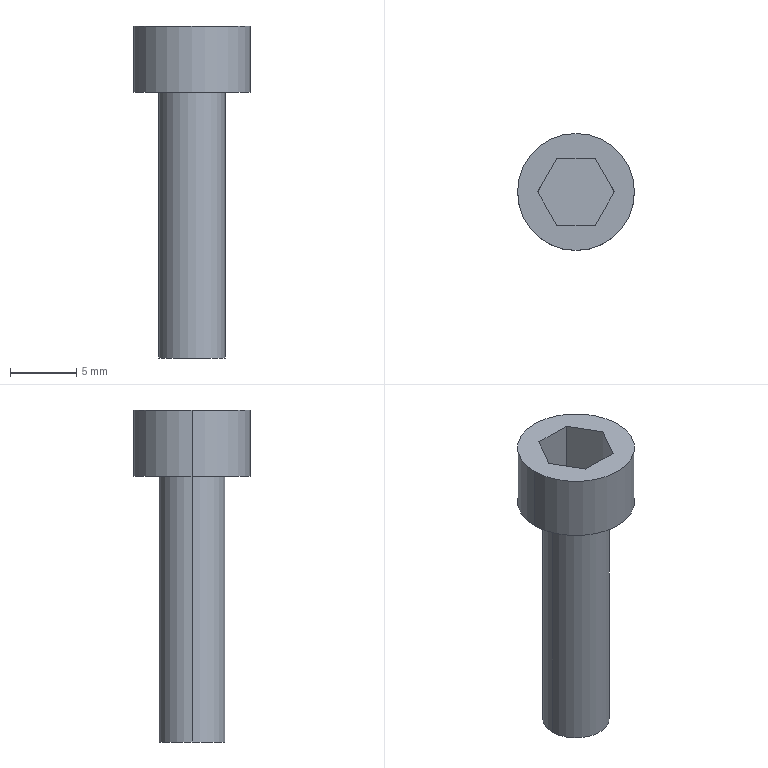Part | STEP file | M5 screw | 1 solid | 14 faces | box 8.8 x 8.8 x 25 mm | volume 610.203 mm3 | plane 10 | cylinder 4 | commonest cylinder face diameters 5 x2 8.8 x2
STEP:
#1=CARTESIAN_POINT('',(0.,0.,0.));
#2=DIRECTION('',(0.,0.,1.));
#3=DIRECTION('',(1.,0.,0.));
#4=AXIS2_PLACEMENT_3D('',#1,#2,#3);
#5=CARTESIAN_POINT('',(4.4,0.,25.));
#6=VERTEX_POINT('',#5);
#7=CARTESIAN_POINT('',(-4.4,0.,25.));
#8=VERTEX_POINT('',#7);
#9=CARTESIAN_POINT('',(0.,0.,25.));
#10=DIRECTION('',(0.,0.,1.));
#11=DIRECTION('',(1.,0.,0.));
#12=AXIS2_PLACEMENT_3D('',#9,#10,#11);
#13=CIRCLE('',#12,4.4);
#14=CARTESIAN_POINT('',(0.,0.,25.));
#15=DIRECTION('',(0.,0.,-1.));
#16=DIRECTION('',(-1.,0.,0.));
#17=AXIS2_PLACEMENT_3D('',#14,#15,#16);
#18=CYLINDRICAL_SURFACE('',#17,4.4);
#19=CARTESIAN_POINT('',(3.142,0.));
#20=DIRECTION('',(-1.,0.));
#21=VECTOR('',#20,1.);
#22=LINE('',#19,#21);
#23=(GEOMETRIC_REPRESENTATION_CONTEXT(2)PARAMETRIC_REPRESENTATION_CONTEXT()REPRESENTATION_CONTEXT('',''));
#24=DEFINITIONAL_REPRESENTATION('',(#22),#23);
#25=PCURVE('',#18,#24);
#26=CARTESIAN_POINT('',(0.,0.,25.));
#27=DIRECTION('',(0.,0.,1.));
#28=DIRECTION('',(1.,0.,0.));
#29=AXIS2_PLACEMENT_3D('',#26,#27,#28);
#30=PLANE('',#29);
#31=CARTESIAN_POINT('',(0.,0.));
#32=DIRECTION('',(1.,0.));
#33=AXIS2_PLACEMENT_2D('',#31,#32);
#34=CIRCLE('',#33,4.4);
#35=(GEOMETRIC_REPRESENTATION_CONTEXT(2)PARAMETRIC_REPRESENTATION_CONTEXT()REPRESENTATION_CONTEXT('',''));
#36=DEFINITIONAL_REPRESENTATION('',(#34),#35);
#37=PCURVE('',#30,#36);
#38=SURFACE_CURVE('',#13,(#25,#37),.PCURVE_S1.);
#39=EDGE_CURVE('',#6,#8,#38,.T.);
#40=ORIENTED_EDGE('',*,*,#39,.F.);
#41=CARTESIAN_POINT('',(4.4,0.,20.));
#42=VERTEX_POINT('',#41);
#43=CARTESIAN_POINT('',(4.4,0.,25.));
#44=DIRECTION('',(0.,0.,-1.));
#45=VECTOR('',#44,1.);
#46=LINE('',#43,#45);
#47=CARTESIAN_POINT('',(3.142,0.));
#48=DIRECTION('',(0.,1.));
#49=VECTOR('',#48,1.);
#50=LINE('',#47,#49);
#51=(GEOMETRIC_REPRESENTATION_CONTEXT(2)PARAMETRIC_REPRESENTATION_CONTEXT()REPRESENTATION_CONTEXT('',''));
#52=DEFINITIONAL_REPRESENTATION('',(#50),#51);
#53=PCURVE('',#18,#52);
#54=CARTESIAN_POINT('',(0.,0.,25.));
#55=DIRECTION('',(0.,0.,-1.));
#56=DIRECTION('',(-1.,0.,0.));
#57=AXIS2_PLACEMENT_3D('',#54,#55,#56);
#58=CYLINDRICAL_SURFACE('',#57,4.4);
#59=CARTESIAN_POINT('',(3.142,0.));
#60=DIRECTION('',(0.,1.));
#61=VECTOR('',#60,1.);
#62=LINE('',#59,#61);
#63=(GEOMETRIC_REPRESENTATION_CONTEXT(2)PARAMETRIC_REPRESENTATION_CONTEXT()REPRESENTATION_CONTEXT('',''));
#64=DEFINITIONAL_REPRESENTATION('',(#62),#63);
#65=PCURVE('',#58,#64);
#66=SURFACE_CURVE('',#46,(#53,#65),.PCURVE_S1.);
#67=EDGE_CURVE('',#6,#42,#66,.T.);
#68=ORIENTED_EDGE('',*,*,#67,.T.);
#69=CARTESIAN_POINT('',(-4.4,0.,20.));
#70=VERTEX_POINT('',#69);
#71=CARTESIAN_POINT('',(0.,0.,20.));
#72=DIRECTION('',(0.,0.,1.));
#73=DIRECTION('',(1.,0.,0.));
#74=AXIS2_PLACEMENT_3D('',#71,#72,#73);
#75=CIRCLE('',#74,4.4);
#76=CARTESIAN_POINT('',(3.142,5.));
#77=DIRECTION('',(-1.,0.));
#78=VECTOR('',#77,1.);
#79=LINE('',#76,#78);
#80=(GEOMETRIC_REPRESENTATION_CONTEXT(2)PARAMETRIC_REPRESENTATION_CONTEXT()REPRESENTATION_CONTEXT('',''));
#81=DEFINITIONAL_REPRESENTATION('',(#79),#80);
#82=PCURVE('',#18,#81);
#83=CARTESIAN_POINT('',(0.,0.,20.));
#84=DIRECTION('',(0.,0.,1.));
#85=DIRECTION('',(1.,0.,0.));
#86=AXIS2_PLACEMENT_3D('',#83,#84,#85);
#87=PLANE('',#86);
#88=CARTESIAN_POINT('',(0.,0.));
#89=DIRECTION('',(1.,0.));
#90=AXIS2_PLACEMENT_2D('',#88,#89);
#91=CIRCLE('',#90,4.4);
#92=(GEOMETRIC_REPRESENTATION_CONTEXT(2)PARAMETRIC_REPRESENTATION_CONTEXT()REPRESENTATION_CONTEXT('',''));
#93=DEFINITIONAL_REPRESENTATION('',(#91),#92);
#94=PCURVE('',#87,#93);
#95=SURFACE_CURVE('',#75,(#82,#94),.PCURVE_S1.);
#96=EDGE_CURVE('',#42,#70,#95,.T.);
#97=ORIENTED_EDGE('',*,*,#96,.T.);
#98=CARTESIAN_POINT('',(-4.4,0.,25.));
#99=DIRECTION('',(0.,0.,-1.));
#100=VECTOR('',#99,1.);
#101=LINE('',#98,#100);
#102=CARTESIAN_POINT('',(0.,0.));
#103=DIRECTION('',(0.,1.));
#104=VECTOR('',#103,1.);
#105=LINE('',#102,#104);
#106=(GEOMETRIC_REPRESENTATION_CONTEXT(2)PARAMETRIC_REPRESENTATION_CONTEXT()REPRESENTATION_CONTEXT('',''));
#107=DEFINITIONAL_REPRESENTATION('',(#105),#106);
#108=PCURVE('',#18,#107);
#109=CARTESIAN_POINT('',(6.283,0.));
#110=DIRECTION('',(0.,1.));
#111=VECTOR('',#110,1.);
#112=LINE('',#109,#111);
#113=(GEOMETRIC_REPRESENTATION_CONTEXT(2)PARAMETRIC_REPRESENTATION_CONTEXT()REPRESENTATION_CONTEXT('',''));
#114=DEFINITIONAL_REPRESENTATION('',(#112),#113);
#115=PCURVE('',#58,#114);
#116=SURFACE_CURVE('',#101,(#108,#115),.PCURVE_S1.);
#117=EDGE_CURVE('',#8,#70,#116,.T.);
#118=ORIENTED_EDGE('',*,*,#117,.F.);
#119=EDGE_LOOP('',(#40,#68,#97,#118));
#120=FACE_BOUND('',#119,.T.);
#121=ADVANCED_FACE('',(#120),#18,.T.);
#122=CARTESIAN_POINT('',(2.5,0.,20.));
#123=VERTEX_POINT('',#122);
#124=CARTESIAN_POINT('',(-2.5,0.,20.));
#125=VERTEX_POINT('',#124);
#126=CARTESIAN_POINT('',(0.,0.,20.));
#127=DIRECTION('',(0.,0.,1.));
#128=DIRECTION('',(1.,0.,0.));
#129=AXIS2_PLACEMENT_3D('',#126,#127,#128);
#130=CIRCLE('',#129,2.5);
#131=CARTESIAN_POINT('',(0.,0.,20.));
#132=DIRECTION('',(0.,0.,-1.));
#133=DIRECTION('',(-1.,0.,0.));
#134=AXIS2_PLACEMENT_3D('',#131,#132,#133);
#135=CYLINDRICAL_SURFACE('',#134,2.5);
#136=CARTESIAN_POINT('',(3.142,0.));
#137=DIRECTION('',(-1.,0.));
#138=VECTOR('',#137,1.);
#139=LINE('',#136,#138);
#140=(GEOMETRIC_REPRESENTATION_CONTEXT(2)PARAMETRIC_REPRESENTATION_CONTEXT()REPRESENTATION_CONTEXT('',''));
#141=DEFINITIONAL_REPRESENTATION('',(#139),#140);
#142=PCURVE('',#135,#141);
#143=CARTESIAN_POINT('',(0.,0.));
#144=DIRECTION('',(1.,0.));
#145=AXIS2_PLACEMENT_2D('',#143,#144);
#146=CIRCLE('',#145,2.5);
#147=(GEOMETRIC_REPRESENTATION_CONTEXT(2)PARAMETRIC_REPRESENTATION_CONTEXT()REPRESENTATION_CONTEXT('',''));
#148=DEFINITIONAL_REPRESENTATION('',(#146),#147);
#149=PCURVE('',#87,#148);
#150=SURFACE_CURVE('',#130,(#142,#149),.PCURVE_S1.);
#151=EDGE_CURVE('',#123,#125,#150,.T.);
#152=ORIENTED_EDGE('',*,*,#151,.F.);
#153=CARTESIAN_POINT('',(2.5,0.,0.));
#154=VERTEX_POINT('',#153);
#155=CARTESIAN_POINT('',(2.5,0.,20.));
#156=DIRECTION('',(0.,0.,-1.));
#157=VECTOR('',#156,1.);
#158=LINE('',#155,#157);
#159=CARTESIAN_POINT('',(3.142,0.));
#160=DIRECTION('',(0.,1.));
#161=VECTOR('',#160,1.);
#162=LINE('',#159,#161);
#163=(GEOMETRIC_REPRESENTATION_CONTEXT(2)PARAMETRIC_REPRESENTATION_CONTEXT()REPRESENTATION_CONTEXT('',''));
#164=DEFINITIONAL_REPRESENTATION('',(#162),#163);
#165=PCURVE('',#135,#164);
#166=CARTESIAN_POINT('',(0.,0.,20.));
#167=DIRECTION('',(0.,0.,-1.));
#168=DIRECTION('',(-1.,0.,0.));
#169=AXIS2_PLACEMENT_3D('',#166,#167,#168);
#170=CYLINDRICAL_SURFACE('',#169,2.5);
#171=CARTESIAN_POINT('',(3.142,0.));
#172=DIRECTION('',(0.,1.));
#173=VECTOR('',#172,1.);
#174=LINE('',#171,#173);
#175=(GEOMETRIC_REPRESENTATION_CONTEXT(2)PARAMETRIC_REPRESENTATION_CONTEXT()REPRESENTATION_CONTEXT('',''));
#176=DEFINITIONAL_REPRESENTATION('',(#174),#175);
#177=PCURVE('',#170,#176);
#178=SURFACE_CURVE('',#158,(#165,#177),.PCURVE_S1.);
#179=EDGE_CURVE('',#123,#154,#178,.T.);
#180=ORIENTED_EDGE('',*,*,#179,.T.);
#181=CARTESIAN_POINT('',(-2.5,0.,0.));
#182=VERTEX_POINT('',#181);
#183=CARTESIAN_POINT('',(0.,0.,0.));
#184=DIRECTION('',(0.,0.,1.));
#185=DIRECTION('',(1.,0.,0.));
#186=AXIS2_PLACEMENT_3D('',#183,#184,#185);
#187=CIRCLE('',#186,2.5);
#188=CARTESIAN_POINT('',(3.142,20.));
#189=DIRECTION('',(-1.,0.));
#190=VECTOR('',#189,1.);
#191=LINE('',#188,#190);
#192=(GEOMETRIC_REPRESENTATION_CONTEXT(2)PARAMETRIC_REPRESENTATION_CONTEXT()REPRESENTATION_CONTEXT('',''));
#193=DEFINITIONAL_REPRESENTATION('',(#191),#192);
#194=PCURVE('',#135,#193);
#195=CARTESIAN_POINT('',(0.,0.,0.));
#196=DIRECTION('',(0.,0.,1.));
#197=DIRECTION('',(1.,0.,0.));
#198=AXIS2_PLACEMENT_3D('',#195,#196,#197);
#199=PLANE('',#198);
#200=CARTESIAN_POINT('',(0.,0.));
#201=DIRECTION('',(1.,0.));
#202=AXIS2_PLACEMENT_2D('',#200,#201);
#203=CIRCLE('',#202,2.5);
#204=(GEOMETRIC_REPRESENTATION_CONTEXT(2)PARAMETRIC_REPRESENTATION_CONTEXT()REPRESENTATION_CONTEXT('',''));
#205=DEFINITIONAL_REPRESENTATION('',(#203),#204);
#206=PCURVE('',#199,#205);
#207=SURFACE_CURVE('',#187,(#194,#206),.PCURVE_S1.);
#208=EDGE_CURVE('',#154,#182,#207,.T.);
#209=ORIENTED_EDGE('',*,*,#208,.T.);
#210=CARTESIAN_POINT('',(-2.5,0.,20.));
#211=DIRECTION('',(0.,0.,-1.));
#212=VECTOR('',#211,1.);
#213=LINE('',#210,#212);
#214=CARTESIAN_POINT('',(0.,0.));
#215=DIRECTION('',(0.,1.));
#216=VECTOR('',#215,1.);
#217=LINE('',#214,#216);
#218=(GEOMETRIC_REPRESENTATION_CONTEXT(2)PARAMETRIC_REPRESENTATION_CONTEXT()REPRESENTATION_CONTEXT('',''));
#219=DEFINITIONAL_REPRESENTATION('',(#217),#218);
#220=PCURVE('',#135,#219);
#221=CARTESIAN_POINT('',(6.283,0.));
#222=DIRECTION('',(0.,1.));
#223=VECTOR('',#222,1.);
#224=LINE('',#221,#223);
#225=(GEOMETRIC_REPRESENTATION_CONTEXT(2)PARAMETRIC_REPRESENTATION_CONTEXT()REPRESENTATION_CONTEXT('',''));
#226=DEFINITIONAL_REPRESENTATION('',(#224),#225);
#227=PCURVE('',#170,#226);
#228=SURFACE_CURVE('',#213,(#220,#227),.PCURVE_S1.);
#229=EDGE_CURVE('',#125,#182,#228,.T.);
#230=ORIENTED_EDGE('',*,*,#229,.F.);
#231=EDGE_LOOP('',(#152,#180,#209,#230));
#232=FACE_BOUND('',#231,.T.);
#233=ADVANCED_FACE('',(#232),#135,.T.);
#234=ORIENTED_EDGE('',*,*,#179,.F.);
#235=CARTESIAN_POINT('',(0.,0.,20.));
#236=DIRECTION('',(0.,0.,1.));
#237=DIRECTION('',(1.,0.,0.));
#238=AXIS2_PLACEMENT_3D('',#235,#236,#237);
#239=CIRCLE('',#238,2.5);
#240=CARTESIAN_POINT('',(9.425,0.));
#241=DIRECTION('',(-1.,0.));
#242=VECTOR('',#241,1.);
#243=LINE('',#240,#242);
#244=(GEOMETRIC_REPRESENTATION_CONTEXT(2)PARAMETRIC_REPRESENTATION_CONTEXT()REPRESENTATION_CONTEXT('',''));
#245=DEFINITIONAL_REPRESENTATION('',(#243),#244);
#246=PCURVE('',#170,#245);
#247=CARTESIAN_POINT('',(0.,0.));
#248=DIRECTION('',(1.,0.));
#249=AXIS2_PLACEMENT_2D('',#247,#248);
#250=CIRCLE('',#249,2.5);
#251=(GEOMETRIC_REPRESENTATION_CONTEXT(2)PARAMETRIC_REPRESENTATION_CONTEXT()REPRESENTATION_CONTEXT('',''));
#252=DEFINITIONAL_REPRESENTATION('',(#250),#251);
#253=PCURVE('',#87,#252);
#254=SURFACE_CURVE('',#239,(#246,#253),.PCURVE_S1.);
#255=EDGE_CURVE('',#125,#123,#254,.T.);
#256=ORIENTED_EDGE('',*,*,#255,.F.);
#257=ORIENTED_EDGE('',*,*,#229,.T.);
#258=CARTESIAN_POINT('',(0.,0.,0.));
#259=DIRECTION('',(0.,0.,1.));
#260=DIRECTION('',(1.,0.,0.));
#261=AXIS2_PLACEMENT_3D('',#258,#259,#260);
#262=CIRCLE('',#261,2.5);
#263=CARTESIAN_POINT('',(9.425,20.));
#264=DIRECTION('',(-1.,0.));
#265=VECTOR('',#264,1.);
#266=LINE('',#263,#265);
#267=(GEOMETRIC_REPRESENTATION_CONTEXT(2)PARAMETRIC_REPRESENTATION_CONTEXT()REPRESENTATION_CONTEXT('',''));
#268=DEFINITIONAL_REPRESENTATION('',(#266),#267);
#269=PCURVE('',#170,#268);
#270=CARTESIAN_POINT('',(0.,0.));
#271=DIRECTION('',(1.,0.));
#272=AXIS2_PLACEMENT_2D('',#270,#271);
#273=CIRCLE('',#272,2.5);
#274=(GEOMETRIC_REPRESENTATION_CONTEXT(2)PARAMETRIC_REPRESENTATION_CONTEXT()REPRESENTATION_CONTEXT('',''));
#275=DEFINITIONAL_REPRESENTATION('',(#273),#274);
#276=PCURVE('',#199,#275);
#277=SURFACE_CURVE('',#262,(#269,#276),.PCURVE_S1.);
#278=EDGE_CURVE('',#182,#154,#277,.T.);
#279=ORIENTED_EDGE('',*,*,#278,.T.);
#280=EDGE_LOOP('',(#234,#256,#257,#279));
#281=FACE_BOUND('',#280,.T.);
#282=ADVANCED_FACE('',(#281),#170,.T.);
#283=ORIENTED_EDGE('',*,*,#278,.F.);
#284=ORIENTED_EDGE('',*,*,#208,.F.);
#285=EDGE_LOOP('',(#283,#284));
#286=FACE_BOUND('',#285,.T.);
#287=ADVANCED_FACE('',(#286),#199,.F.);
#288=CARTESIAN_POINT('',(0.,0.,20.));
#289=DIRECTION('',(0.,0.,1.));
#290=DIRECTION('',(1.,0.,0.));
#291=AXIS2_PLACEMENT_3D('',#288,#289,#290);
#292=CIRCLE('',#291,4.4);
#293=CARTESIAN_POINT('',(0.,0.));
#294=DIRECTION('',(1.,0.));
#295=AXIS2_PLACEMENT_2D('',#293,#294);
#296=CIRCLE('',#295,4.4);
#297=(GEOMETRIC_REPRESENTATION_CONTEXT(2)PARAMETRIC_REPRESENTATION_CONTEXT()REPRESENTATION_CONTEXT('',''));
#298=DEFINITIONAL_REPRESENTATION('',(#296),#297);
#299=PCURVE('',#87,#298);
#300=CARTESIAN_POINT('',(9.425,5.));
#301=DIRECTION('',(-1.,0.));
#302=VECTOR('',#301,1.);
#303=LINE('',#300,#302);
#304=(GEOMETRIC_REPRESENTATION_CONTEXT(2)PARAMETRIC_REPRESENTATION_CONTEXT()REPRESENTATION_CONTEXT('',''));
#305=DEFINITIONAL_REPRESENTATION('',(#303),#304);
#306=PCURVE('',#58,#305);
#307=SURFACE_CURVE('',#292,(#299,#306),.PCURVE_S1.);
#308=EDGE_CURVE('',#70,#42,#307,.T.);
#309=ORIENTED_EDGE('',*,*,#308,.F.);
#310=ORIENTED_EDGE('',*,*,#96,.F.);
#311=EDGE_LOOP('',(#309,#310));
#312=FACE_BOUND('',#311,.T.);
#313=ORIENTED_EDGE('',*,*,#255,.T.);
#314=ORIENTED_EDGE('',*,*,#151,.T.);
#315=EDGE_LOOP('',(#313,#314));
#316=FACE_BOUND('',#315,.T.);
#317=ADVANCED_FACE('',(#312,#316),#87,.F.);
#318=ORIENTED_EDGE('',*,*,#67,.F.);
#319=CARTESIAN_POINT('',(0.,0.,25.));
#320=DIRECTION('',(0.,0.,1.));
#321=DIRECTION('',(1.,0.,0.));
#322=AXIS2_PLACEMENT_3D('',#319,#320,#321);
#323=CIRCLE('',#322,4.4);
#324=CARTESIAN_POINT('',(9.425,0.));
#325=DIRECTION('',(-1.,0.));
#326=VECTOR('',#325,1.);
#327=LINE('',#324,#326);
#328=(GEOMETRIC_REPRESENTATION_CONTEXT(2)PARAMETRIC_REPRESENTATION_CONTEXT()REPRESENTATION_CONTEXT('',''));
#329=DEFINITIONAL_REPRESENTATION('',(#327),#328);
#330=PCURVE('',#58,#329);
#331=CARTESIAN_POINT('',(0.,0.));
#332=DIRECTION('',(1.,0.));
#333=AXIS2_PLACEMENT_2D('',#331,#332);
#334=CIRCLE('',#333,4.4);
#335=(GEOMETRIC_REPRESENTATION_CONTEXT(2)PARAMETRIC_REPRESENTATION_CONTEXT()REPRESENTATION_CONTEXT('',''));
#336=DEFINITIONAL_REPRESENTATION('',(#334),#335);
#337=PCURVE('',#30,#336);
#338=SURFACE_CURVE('',#323,(#330,#337),.PCURVE_S1.);
#339=EDGE_CURVE('',#8,#6,#338,.T.);
#340=ORIENTED_EDGE('',*,*,#339,.F.);
#341=ORIENTED_EDGE('',*,*,#117,.T.);
#342=ORIENTED_EDGE('',*,*,#308,.T.);
#343=EDGE_LOOP('',(#318,#340,#341,#342));
#344=FACE_BOUND('',#343,.T.);
#345=ADVANCED_FACE('',(#344),#58,.T.);
#346=CARTESIAN_POINT('',(2.887,0.,25.));
#347=VERTEX_POINT('',#346);
#348=CARTESIAN_POINT('',(1.443,2.5,25.));
#349=VERTEX_POINT('',#348);
#350=CARTESIAN_POINT('',(2.887,0.,25.));
#351=DIRECTION('',(-0.5,0.866,0.));
#352=VECTOR('',#351,1.);
#353=LINE('',#350,#352);
#354=CARTESIAN_POINT('',(2.887,0.));
#355=DIRECTION('',(-0.5,0.866));
#356=VECTOR('',#355,1.);
#357=LINE('',#354,#356);
#358=(GEOMETRIC_REPRESENTATION_CONTEXT(2)PARAMETRIC_REPRESENTATION_CONTEXT()REPRESENTATION_CONTEXT('',''));
#359=DEFINITIONAL_REPRESENTATION('',(#357),#358);
#360=PCURVE('',#30,#359);
#361=CARTESIAN_POINT('',(2.887,0.,21.));
#362=DIRECTION('',(0.866,0.5,0.));
#363=DIRECTION('',(-0.5,0.866,0.));
#364=AXIS2_PLACEMENT_3D('',#361,#362,#363);
#365=PLANE('',#364);
#366=CARTESIAN_POINT('',(0.,4.));
#367=DIRECTION('',(1.,0.));
#368=VECTOR('',#367,1.);
#369=LINE('',#366,#368);
#370=(GEOMETRIC_REPRESENTATION_CONTEXT(2)PARAMETRIC_REPRESENTATION_CONTEXT()REPRESENTATION_CONTEXT('',''));
#371=DEFINITIONAL_REPRESENTATION('',(#369),#370);
#372=PCURVE('',#365,#371);
#373=SURFACE_CURVE('',#353,(#360,#372),.PCURVE_S1.);
#374=EDGE_CURVE('',#347,#349,#373,.T.);
#375=ORIENTED_EDGE('',*,*,#374,.F.);
#376=CARTESIAN_POINT('',(1.443,-2.5,25.));
#377=VERTEX_POINT('',#376);
#378=CARTESIAN_POINT('',(1.443,-2.5,25.));
#379=DIRECTION('',(0.5,0.866,0.));
#380=VECTOR('',#379,1.);
#381=LINE('',#378,#380);
#382=CARTESIAN_POINT('',(1.443,-2.5));
#383=DIRECTION('',(0.5,0.866));
#384=VECTOR('',#383,1.);
#385=LINE('',#382,#384);
#386=(GEOMETRIC_REPRESENTATION_CONTEXT(2)PARAMETRIC_REPRESENTATION_CONTEXT()REPRESENTATION_CONTEXT('',''));
#387=DEFINITIONAL_REPRESENTATION('',(#385),#386);
#388=PCURVE('',#30,#387);
#389=CARTESIAN_POINT('',(1.443,-2.5,21.));
#390=DIRECTION('',(0.866,-0.5,0.));
#391=DIRECTION('',(0.5,0.866,0.));
#392=AXIS2_PLACEMENT_3D('',#389,#390,#391);
#393=PLANE('',#392);
#394=CARTESIAN_POINT('',(0.,4.));
#395=DIRECTION('',(1.,0.));
#396=VECTOR('',#395,1.);
#397=LINE('',#394,#396);
#398=(GEOMETRIC_REPRESENTATION_CONTEXT(2)PARAMETRIC_REPRESENTATION_CONTEXT()REPRESENTATION_CONTEXT('',''));
#399=DEFINITIONAL_REPRESENTATION('',(#397),#398);
#400=PCURVE('',#393,#399);
#401=SURFACE_CURVE('',#381,(#388,#400),.PCURVE_S1.);
#402=EDGE_CURVE('',#377,#347,#401,.T.);
#403=ORIENTED_EDGE('',*,*,#402,.F.);
#404=CARTESIAN_POINT('',(-1.443,-2.5,25.));
#405=VERTEX_POINT('',#404);
#406=CARTESIAN_POINT('',(-1.443,-2.5,25.));
#407=DIRECTION('',(1.,0.,0.));
#408=VECTOR('',#407,1.);
#409=LINE('',#406,#408);
#410=CARTESIAN_POINT('',(-1.443,-2.5));
#411=DIRECTION('',(1.,0.));
#412=VECTOR('',#411,1.);
#413=LINE('',#410,#412);
#414=(GEOMETRIC_REPRESENTATION_CONTEXT(2)PARAMETRIC_REPRESENTATION_CONTEXT()REPRESENTATION_CONTEXT('',''));
#415=DEFINITIONAL_REPRESENTATION('',(#413),#414);
#416=PCURVE('',#30,#415);
#417=CARTESIAN_POINT('',(-1.443,-2.5,21.));
#418=DIRECTION('',(0.,-1.,0.));
#419=DIRECTION('',(1.,0.,0.));
#420=AXIS2_PLACEMENT_3D('',#417,#418,#419);
#421=PLANE('',#420);
#422=CARTESIAN_POINT('',(0.,4.));
#423=DIRECTION('',(1.,0.));
#424=VECTOR('',#423,1.);
#425=LINE('',#422,#424);
#426=(GEOMETRIC_REPRESENTATION_CONTEXT(2)PARAMETRIC_REPRESENTATION_CONTEXT()REPRESENTATION_CONTEXT('',''));
#427=DEFINITIONAL_REPRESENTATION('',(#425),#426);
#428=PCURVE('',#421,#427);
#429=SURFACE_CURVE('',#409,(#416,#428),.PCURVE_S1.);
#430=EDGE_CURVE('',#405,#377,#429,.T.);
#431=ORIENTED_EDGE('',*,*,#430,.F.);
#432=CARTESIAN_POINT('',(-2.887,0.,25.));
#433=VERTEX_POINT('',#432);
#434=CARTESIAN_POINT('',(-2.887,0.,25.));
#435=DIRECTION('',(0.5,-0.866,0.));
#436=VECTOR('',#435,1.);
#437=LINE('',#434,#436);
#438=CARTESIAN_POINT('',(-2.887,0.));
#439=DIRECTION('',(0.5,-0.866));
#440=VECTOR('',#439,1.);
#441=LINE('',#438,#440);
#442=(GEOMETRIC_REPRESENTATION_CONTEXT(2)PARAMETRIC_REPRESENTATION_CONTEXT()REPRESENTATION_CONTEXT('',''));
#443=DEFINITIONAL_REPRESENTATION('',(#441),#442);
#444=PCURVE('',#30,#443);
#445=CARTESIAN_POINT('',(-2.887,0.,21.));
#446=DIRECTION('',(-0.866,-0.5,0.));
#447=DIRECTION('',(0.5,-0.866,0.));
#448=AXIS2_PLACEMENT_3D('',#445,#446,#447);
#449=PLANE('',#448);
#450=CARTESIAN_POINT('',(0.,4.));
#451=DIRECTION('',(1.,0.));
#452=VECTOR('',#451,1.);
#453=LINE('',#450,#452);
#454=(GEOMETRIC_REPRESENTATION_CONTEXT(2)PARAMETRIC_REPRESENTATION_CONTEXT()REPRESENTATION_CONTEXT('',''));
#455=DEFINITIONAL_REPRESENTATION('',(#453),#454);
#456=PCURVE('',#449,#455);
#457=SURFACE_CURVE('',#437,(#444,#456),.PCURVE_S1.);
#458=EDGE_CURVE('',#433,#405,#457,.T.);
#459=ORIENTED_EDGE('',*,*,#458,.F.);
#460=CARTESIAN_POINT('',(-1.443,2.5,25.));
#461=VERTEX_POINT('',#460);
#462=CARTESIAN_POINT('',(-1.443,2.5,25.));
#463=DIRECTION('',(-0.5,-0.866,0.));
#464=VECTOR('',#463,1.);
#465=LINE('',#462,#464);
#466=CARTESIAN_POINT('',(-1.443,2.5));
#467=DIRECTION('',(-0.5,-0.866));
#468=VECTOR('',#467,1.);
#469=LINE('',#466,#468);
#470=(GEOMETRIC_REPRESENTATION_CONTEXT(2)PARAMETRIC_REPRESENTATION_CONTEXT()REPRESENTATION_CONTEXT('',''));
#471=DEFINITIONAL_REPRESENTATION('',(#469),#470);
#472=PCURVE('',#30,#471);
#473=CARTESIAN_POINT('',(-1.443,2.5,21.));
#474=DIRECTION('',(-0.866,0.5,0.));
#475=DIRECTION('',(-0.5,-0.866,0.));
#476=AXIS2_PLACEMENT_3D('',#473,#474,#475);
#477=PLANE('',#476);
#478=CARTESIAN_POINT('',(0.,4.));
#479=DIRECTION('',(1.,0.));
#480=VECTOR('',#479,1.);
#481=LINE('',#478,#480);
#482=(GEOMETRIC_REPRESENTATION_CONTEXT(2)PARAMETRIC_REPRESENTATION_CONTEXT()REPRESENTATION_CONTEXT('',''));
#483=DEFINITIONAL_REPRESENTATION('',(#481),#482);
#484=PCURVE('',#477,#483);
#485=SURFACE_CURVE('',#465,(#472,#484),.PCURVE_S1.);
#486=EDGE_CURVE('',#461,#433,#485,.T.);
#487=ORIENTED_EDGE('',*,*,#486,.F.);
#488=CARTESIAN_POINT('',(1.443,2.5,25.));
#489=DIRECTION('',(-1.,0.,0.));
#490=VECTOR('',#489,1.);
#491=LINE('',#488,#490);
#492=CARTESIAN_POINT('',(1.443,2.5));
#493=DIRECTION('',(-1.,0.));
#494=VECTOR('',#493,1.);
#495=LINE('',#492,#494);
#496=(GEOMETRIC_REPRESENTATION_CONTEXT(2)PARAMETRIC_REPRESENTATION_CONTEXT()REPRESENTATION_CONTEXT('',''));
#497=DEFINITIONAL_REPRESENTATION('',(#495),#496);
#498=PCURVE('',#30,#497);
#499=CARTESIAN_POINT('',(1.443,2.5,21.));
#500=DIRECTION('',(0.,1.,0.));
#501=DIRECTION('',(0.,0.,1.));
#502=AXIS2_PLACEMENT_3D('',#499,#500,#501);
#503=PLANE('',#502);
#504=CARTESIAN_POINT('',(4.,0.));
#505=DIRECTION('',(0.,-1.));
#506=VECTOR('',#505,1.);
#507=LINE('',#504,#506);
#508=(GEOMETRIC_REPRESENTATION_CONTEXT(2)PARAMETRIC_REPRESENTATION_CONTEXT()REPRESENTATION_CONTEXT('',''));
#509=DEFINITIONAL_REPRESENTATION('',(#507),#508);
#510=PCURVE('',#503,#509);
#511=SURFACE_CURVE('',#491,(#498,#510),.PCURVE_S1.);
#512=EDGE_CURVE('',#349,#461,#511,.T.);
#513=ORIENTED_EDGE('',*,*,#512,.F.);
#514=EDGE_LOOP('',(#375,#403,#431,#459,#487,#513));
#515=FACE_BOUND('',#514,.T.);
#516=ORIENTED_EDGE('',*,*,#339,.T.);
#517=ORIENTED_EDGE('',*,*,#39,.T.);
#518=EDGE_LOOP('',(#516,#517));
#519=FACE_BOUND('',#518,.T.);
#520=ADVANCED_FACE('',(#515,#519),#30,.T.);
#521=ORIENTED_EDGE('',*,*,#374,.T.);
#522=CARTESIAN_POINT('',(1.443,2.5,21.));
#523=VERTEX_POINT('',#522);
#524=CARTESIAN_POINT('',(1.443,2.5,21.));
#525=DIRECTION('',(0.,0.,1.));
#526=VECTOR('',#525,1.);
#527=LINE('',#524,#526);
#528=CARTESIAN_POINT('',(2.887,0.));
#529=DIRECTION('',(0.,1.));
#530=VECTOR('',#529,1.);
#531=LINE('',#528,#530);
#532=(GEOMETRIC_REPRESENTATION_CONTEXT(2)PARAMETRIC_REPRESENTATION_CONTEXT()REPRESENTATION_CONTEXT('',''));
#533=DEFINITIONAL_REPRESENTATION('',(#531),#532);
#534=PCURVE('',#365,#533);
#535=CARTESIAN_POINT('',(0.,0.));
#536=DIRECTION('',(1.,0.));
#537=VECTOR('',#536,1.);
#538=LINE('',#535,#537);
#539=(GEOMETRIC_REPRESENTATION_CONTEXT(2)PARAMETRIC_REPRESENTATION_CONTEXT()REPRESENTATION_CONTEXT('',''));
#540=DEFINITIONAL_REPRESENTATION('',(#538),#539);
#541=PCURVE('',#503,#540);
#542=SURFACE_CURVE('',#527,(#534,#541),.PCURVE_S1.);
#543=EDGE_CURVE('',#523,#349,#542,.T.);
#544=ORIENTED_EDGE('',*,*,#543,.F.);
#545=CARTESIAN_POINT('',(2.887,0.,21.));
#546=VERTEX_POINT('',#545);
#547=CARTESIAN_POINT('',(2.887,0.,21.));
#548=DIRECTION('',(-0.5,0.866,0.));
#549=VECTOR('',#548,1.);
#550=LINE('',#547,#549);
#551=CARTESIAN_POINT('',(0.,0.));
#552=DIRECTION('',(1.,0.));
#553=VECTOR('',#552,1.);
#554=LINE('',#551,#553);
#555=(GEOMETRIC_REPRESENTATION_CONTEXT(2)PARAMETRIC_REPRESENTATION_CONTEXT()REPRESENTATION_CONTEXT('',''));
#556=DEFINITIONAL_REPRESENTATION('',(#554),#555);
#557=PCURVE('',#365,#556);
#558=CARTESIAN_POINT('',(0.,0.,21.));
#559=DIRECTION('',(0.,0.,1.));
#560=DIRECTION('',(1.,0.,0.));
#561=AXIS2_PLACEMENT_3D('',#558,#559,#560);
#562=PLANE('',#561);
#563=CARTESIAN_POINT('',(2.887,0.));
#564=DIRECTION('',(-0.5,0.866));
#565=VECTOR('',#564,1.);
#566=LINE('',#563,#565);
#567=(GEOMETRIC_REPRESENTATION_CONTEXT(2)PARAMETRIC_REPRESENTATION_CONTEXT()REPRESENTATION_CONTEXT('',''));
#568=DEFINITIONAL_REPRESENTATION('',(#566),#567);
#569=PCURVE('',#562,#568);
#570=SURFACE_CURVE('',#550,(#557,#569),.PCURVE_S1.);
#571=EDGE_CURVE('',#546,#523,#570,.T.);
#572=ORIENTED_EDGE('',*,*,#571,.F.);
#573=CARTESIAN_POINT('',(2.887,0.,21.));
#574=DIRECTION('',(0.,0.,1.));
#575=VECTOR('',#574,1.);
#576=LINE('',#573,#575);
#577=CARTESIAN_POINT('',(0.,0.));
#578=DIRECTION('',(0.,1.));
#579=VECTOR('',#578,1.);
#580=LINE('',#577,#579);
#581=(GEOMETRIC_REPRESENTATION_CONTEXT(2)PARAMETRIC_REPRESENTATION_CONTEXT()REPRESENTATION_CONTEXT('',''));
#582=DEFINITIONAL_REPRESENTATION('',(#580),#581);
#583=PCURVE('',#365,#582);
#584=CARTESIAN_POINT('',(2.887,0.));
#585=DIRECTION('',(0.,1.));
#586=VECTOR('',#585,1.);
#587=LINE('',#584,#586);
#588=(GEOMETRIC_REPRESENTATION_CONTEXT(2)PARAMETRIC_REPRESENTATION_CONTEXT()REPRESENTATION_CONTEXT('',''));
#589=DEFINITIONAL_REPRESENTATION('',(#587),#588);
#590=PCURVE('',#393,#589);
#591=SURFACE_CURVE('',#576,(#583,#590),.PCURVE_S1.);
#592=EDGE_CURVE('',#546,#347,#591,.T.);
#593=ORIENTED_EDGE('',*,*,#592,.T.);
#594=EDGE_LOOP('',(#521,#544,#572,#593));
#595=FACE_BOUND('',#594,.T.);
#596=ADVANCED_FACE('',(#595),#365,.F.);
#597=ORIENTED_EDGE('',*,*,#402,.T.);
#598=ORIENTED_EDGE('',*,*,#592,.F.);
#599=CARTESIAN_POINT('',(1.443,-2.5,21.));
#600=VERTEX_POINT('',#599);
#601=CARTESIAN_POINT('',(1.443,-2.5,21.));
#602=DIRECTION('',(0.5,0.866,0.));
#603=VECTOR('',#602,1.);
#604=LINE('',#601,#603);
#605=CARTESIAN_POINT('',(0.,0.));
#606=DIRECTION('',(1.,0.));
#607=VECTOR('',#606,1.);
#608=LINE('',#605,#607);
#609=(GEOMETRIC_REPRESENTATION_CONTEXT(2)PARAMETRIC_REPRESENTATION_CONTEXT()REPRESENTATION_CONTEXT('',''));
#610=DEFINITIONAL_REPRESENTATION('',(#608),#609);
#611=PCURVE('',#393,#610);
#612=CARTESIAN_POINT('',(1.443,-2.5));
#613=DIRECTION('',(0.5,0.866));
#614=VECTOR('',#613,1.);
#615=LINE('',#612,#614);
#616=(GEOMETRIC_REPRESENTATION_CONTEXT(2)PARAMETRIC_REPRESENTATION_CONTEXT()REPRESENTATION_CONTEXT('',''));
#617=DEFINITIONAL_REPRESENTATION('',(#615),#616);
#618=PCURVE('',#562,#617);
#619=SURFACE_CURVE('',#604,(#611,#618),.PCURVE_S1.);
#620=EDGE_CURVE('',#600,#546,#619,.T.);
#621=ORIENTED_EDGE('',*,*,#620,.F.);
#622=CARTESIAN_POINT('',(1.443,-2.5,21.));
#623=DIRECTION('',(0.,0.,1.));
#624=VECTOR('',#623,1.);
#625=LINE('',#622,#624);
#626=CARTESIAN_POINT('',(0.,0.));
#627=DIRECTION('',(0.,1.));
#628=VECTOR('',#627,1.);
#629=LINE('',#626,#628);
#630=(GEOMETRIC_REPRESENTATION_CONTEXT(2)PARAMETRIC_REPRESENTATION_CONTEXT()REPRESENTATION_CONTEXT('',''));
#631=DEFINITIONAL_REPRESENTATION('',(#629),#630);
#632=PCURVE('',#393,#631);
#633=CARTESIAN_POINT('',(2.887,0.));
#634=DIRECTION('',(0.,1.));
#635=VECTOR('',#634,1.);
#636=LINE('',#633,#635);
#637=(GEOMETRIC_REPRESENTATION_CONTEXT(2)PARAMETRIC_REPRESENTATION_CONTEXT()REPRESENTATION_CONTEXT('',''));
#638=DEFINITIONAL_REPRESENTATION('',(#636),#637);
#639=PCURVE('',#421,#638);
#640=SURFACE_CURVE('',#625,(#632,#639),.PCURVE_S1.);
#641=EDGE_CURVE('',#600,#377,#640,.T.);
#642=ORIENTED_EDGE('',*,*,#641,.T.);
#643=EDGE_LOOP('',(#597,#598,#621,#642));
#644=FACE_BOUND('',#643,.T.);
#645=ADVANCED_FACE('',(#644),#393,.F.);
#646=ORIENTED_EDGE('',*,*,#430,.T.);
#647=ORIENTED_EDGE('',*,*,#641,.F.);
#648=CARTESIAN_POINT('',(-1.443,-2.5,21.));
#649=VERTEX_POINT('',#648);
#650=CARTESIAN_POINT('',(-1.443,-2.5,21.));
#651=DIRECTION('',(1.,0.,0.));
#652=VECTOR('',#651,1.);
#653=LINE('',#650,#652);
#654=CARTESIAN_POINT('',(0.,0.));
#655=DIRECTION('',(1.,0.));
#656=VECTOR('',#655,1.);
#657=LINE('',#654,#656);
#658=(GEOMETRIC_REPRESENTATION_CONTEXT(2)PARAMETRIC_REPRESENTATION_CONTEXT()REPRESENTATION_CONTEXT('',''));
#659=DEFINITIONAL_REPRESENTATION('',(#657),#658);
#660=PCURVE('',#421,#659);
#661=CARTESIAN_POINT('',(-1.443,-2.5));
#662=DIRECTION('',(1.,0.));
#663=VECTOR('',#662,1.);
#664=LINE('',#661,#663);
#665=(GEOMETRIC_REPRESENTATION_CONTEXT(2)PARAMETRIC_REPRESENTATION_CONTEXT()REPRESENTATION_CONTEXT('',''));
#666=DEFINITIONAL_REPRESENTATION('',(#664),#665);
#667=PCURVE('',#562,#666);
#668=SURFACE_CURVE('',#653,(#660,#667),.PCURVE_S1.);
#669=EDGE_CURVE('',#649,#600,#668,.T.);
#670=ORIENTED_EDGE('',*,*,#669,.F.);
#671=CARTESIAN_POINT('',(-1.443,-2.5,21.));
#672=DIRECTION('',(0.,0.,1.));
#673=VECTOR('',#672,1.);
#674=LINE('',#671,#673);
#675=CARTESIAN_POINT('',(0.,0.));
#676=DIRECTION('',(0.,1.));
#677=VECTOR('',#676,1.);
#678=LINE('',#675,#677);
#679=(GEOMETRIC_REPRESENTATION_CONTEXT(2)PARAMETRIC_REPRESENTATION_CONTEXT()REPRESENTATION_CONTEXT('',''));
#680=DEFINITIONAL_REPRESENTATION('',(#678),#679);
#681=PCURVE('',#421,#680);
#682=CARTESIAN_POINT('',(2.887,0.));
#683=DIRECTION('',(0.,1.));
#684=VECTOR('',#683,1.);
#685=LINE('',#682,#684);
#686=(GEOMETRIC_REPRESENTATION_CONTEXT(2)PARAMETRIC_REPRESENTATION_CONTEXT()REPRESENTATION_CONTEXT('',''));
#687=DEFINITIONAL_REPRESENTATION('',(#685),#686);
#688=PCURVE('',#449,#687);
#689=SURFACE_CURVE('',#674,(#681,#688),.PCURVE_S1.);
#690=EDGE_CURVE('',#649,#405,#689,.T.);
#691=ORIENTED_EDGE('',*,*,#690,.T.);
#692=EDGE_LOOP('',(#646,#647,#670,#691));
#693=FACE_BOUND('',#692,.T.);
#694=ADVANCED_FACE('',(#693),#421,.F.);
#695=ORIENTED_EDGE('',*,*,#458,.T.);
#696=ORIENTED_EDGE('',*,*,#690,.F.);
#697=CARTESIAN_POINT('',(-2.887,0.,21.));
#698=VERTEX_POINT('',#697);
#699=CARTESIAN_POINT('',(-2.887,0.,21.));
#700=DIRECTION('',(0.5,-0.866,0.));
#701=VECTOR('',#700,1.);
#702=LINE('',#699,#701);
#703=CARTESIAN_POINT('',(0.,0.));
#704=DIRECTION('',(1.,0.));
#705=VECTOR('',#704,1.);
#706=LINE('',#703,#705);
#707=(GEOMETRIC_REPRESENTATION_CONTEXT(2)PARAMETRIC_REPRESENTATION_CONTEXT()REPRESENTATION_CONTEXT('',''));
#708=DEFINITIONAL_REPRESENTATION('',(#706),#707);
#709=PCURVE('',#449,#708);
#710=CARTESIAN_POINT('',(-2.887,0.));
#711=DIRECTION('',(0.5,-0.866));
#712=VECTOR('',#711,1.);
#713=LINE('',#710,#712);
#714=(GEOMETRIC_REPRESENTATION_CONTEXT(2)PARAMETRIC_REPRESENTATION_CONTEXT()REPRESENTATION_CONTEXT('',''));
#715=DEFINITIONAL_REPRESENTATION('',(#713),#714);
#716=PCURVE('',#562,#715);
#717=SURFACE_CURVE('',#702,(#709,#716),.PCURVE_S1.);
#718=EDGE_CURVE('',#698,#649,#717,.T.);
#719=ORIENTED_EDGE('',*,*,#718,.F.);
#720=CARTESIAN_POINT('',(-2.887,0.,21.));
#721=DIRECTION('',(0.,0.,1.));
#722=VECTOR('',#721,1.);
#723=LINE('',#720,#722);
#724=CARTESIAN_POINT('',(0.,0.));
#725=DIRECTION('',(0.,1.));
#726=VECTOR('',#725,1.);
#727=LINE('',#724,#726);
#728=(GEOMETRIC_REPRESENTATION_CONTEXT(2)PARAMETRIC_REPRESENTATION_CONTEXT()REPRESENTATION_CONTEXT('',''));
#729=DEFINITIONAL_REPRESENTATION('',(#727),#728);
#730=PCURVE('',#449,#729);
#731=CARTESIAN_POINT('',(2.887,0.));
#732=DIRECTION('',(0.,1.));
#733=VECTOR('',#732,1.);
#734=LINE('',#731,#733);
#735=(GEOMETRIC_REPRESENTATION_CONTEXT(2)PARAMETRIC_REPRESENTATION_CONTEXT()REPRESENTATION_CONTEXT('',''));
#736=DEFINITIONAL_REPRESENTATION('',(#734),#735);
#737=PCURVE('',#477,#736);
#738=SURFACE_CURVE('',#723,(#730,#737),.PCURVE_S1.);
#739=EDGE_CURVE('',#698,#433,#738,.T.);
#740=ORIENTED_EDGE('',*,*,#739,.T.);
#741=EDGE_LOOP('',(#695,#696,#719,#740));
#742=FACE_BOUND('',#741,.T.);
#743=ADVANCED_FACE('',(#742),#449,.F.);
#744=ORIENTED_EDGE('',*,*,#486,.T.);
#745=ORIENTED_EDGE('',*,*,#739,.F.);
#746=CARTESIAN_POINT('',(-1.443,2.5,21.));
#747=VERTEX_POINT('',#746);
#748=CARTESIAN_POINT('',(-1.443,2.5,21.));
#749=DIRECTION('',(-0.5,-0.866,0.));
#750=VECTOR('',#749,1.);
#751=LINE('',#748,#750);
#752=CARTESIAN_POINT('',(0.,0.));
#753=DIRECTION('',(1.,0.));
#754=VECTOR('',#753,1.);
#755=LINE('',#752,#754);
#756=(GEOMETRIC_REPRESENTATION_CONTEXT(2)PARAMETRIC_REPRESENTATION_CONTEXT()REPRESENTATION_CONTEXT('',''));
#757=DEFINITIONAL_REPRESENTATION('',(#755),#756);
#758=PCURVE('',#477,#757);
#759=CARTESIAN_POINT('',(-1.443,2.5));
#760=DIRECTION('',(-0.5,-0.866));
#761=VECTOR('',#760,1.);
#762=LINE('',#759,#761);
#763=(GEOMETRIC_REPRESENTATION_CONTEXT(2)PARAMETRIC_REPRESENTATION_CONTEXT()REPRESENTATION_CONTEXT('',''));
#764=DEFINITIONAL_REPRESENTATION('',(#762),#763);
#765=PCURVE('',#562,#764);
#766=SURFACE_CURVE('',#751,(#758,#765),.PCURVE_S1.);
#767=EDGE_CURVE('',#747,#698,#766,.T.);
#768=ORIENTED_EDGE('',*,*,#767,.F.);
#769=CARTESIAN_POINT('',(-1.443,2.5,21.));
#770=DIRECTION('',(0.,0.,1.));
#771=VECTOR('',#770,1.);
#772=LINE('',#769,#771);
#773=CARTESIAN_POINT('',(0.,0.));
#774=DIRECTION('',(0.,1.));
#775=VECTOR('',#774,1.);
#776=LINE('',#773,#775);
#777=(GEOMETRIC_REPRESENTATION_CONTEXT(2)PARAMETRIC_REPRESENTATION_CONTEXT()REPRESENTATION_CONTEXT('',''));
#778=DEFINITIONAL_REPRESENTATION('',(#776),#777);
#779=PCURVE('',#477,#778);
#780=CARTESIAN_POINT('',(0.,-2.887));
#781=DIRECTION('',(1.,0.));
#782=VECTOR('',#781,1.);
#783=LINE('',#780,#782);
#784=(GEOMETRIC_REPRESENTATION_CONTEXT(2)PARAMETRIC_REPRESENTATION_CONTEXT()REPRESENTATION_CONTEXT('',''));
#785=DEFINITIONAL_REPRESENTATION('',(#783),#784);
#786=PCURVE('',#503,#785);
#787=SURFACE_CURVE('',#772,(#779,#786),.PCURVE_S1.);
#788=EDGE_CURVE('',#747,#461,#787,.T.);
#789=ORIENTED_EDGE('',*,*,#788,.T.);
#790=EDGE_LOOP('',(#744,#745,#768,#789));
#791=FACE_BOUND('',#790,.T.);
#792=ADVANCED_FACE('',(#791),#477,.F.);
#793=ORIENTED_EDGE('',*,*,#512,.T.);
#794=ORIENTED_EDGE('',*,*,#788,.F.);
#795=CARTESIAN_POINT('',(1.443,2.5,21.));
#796=DIRECTION('',(-1.,0.,0.));
#797=VECTOR('',#796,1.);
#798=LINE('',#795,#797);
#799=CARTESIAN_POINT('',(0.,0.));
#800=DIRECTION('',(0.,-1.));
#801=VECTOR('',#800,1.);
#802=LINE('',#799,#801);
#803=(GEOMETRIC_REPRESENTATION_CONTEXT(2)PARAMETRIC_REPRESENTATION_CONTEXT()REPRESENTATION_CONTEXT('',''));
#804=DEFINITIONAL_REPRESENTATION('',(#802),#803);
#805=PCURVE('',#503,#804);
#806=CARTESIAN_POINT('',(1.443,2.5));
#807=DIRECTION('',(-1.,0.));
#808=VECTOR('',#807,1.);
#809=LINE('',#806,#808);
#810=(GEOMETRIC_REPRESENTATION_CONTEXT(2)PARAMETRIC_REPRESENTATION_CONTEXT()REPRESENTATION_CONTEXT('',''));
#811=DEFINITIONAL_REPRESENTATION('',(#809),#810);
#812=PCURVE('',#562,#811);
#813=SURFACE_CURVE('',#798,(#805,#812),.PCURVE_S1.);
#814=EDGE_CURVE('',#523,#747,#813,.T.);
#815=ORIENTED_EDGE('',*,*,#814,.F.);
#816=ORIENTED_EDGE('',*,*,#543,.T.);
#817=EDGE_LOOP('',(#793,#794,#815,#816));
#818=FACE_BOUND('',#817,.T.);
#819=ADVANCED_FACE('',(#818),#503,.F.);
#820=ORIENTED_EDGE('',*,*,#571,.T.);
#821=ORIENTED_EDGE('',*,*,#814,.T.);
#822=ORIENTED_EDGE('',*,*,#767,.T.);
#823=ORIENTED_EDGE('',*,*,#718,.T.);
#824=ORIENTED_EDGE('',*,*,#669,.T.);
#825=ORIENTED_EDGE('',*,*,#620,.T.);
#826=EDGE_LOOP('',(#820,#821,#822,#823,#824,#825));
#827=FACE_BOUND('',#826,.T.);
#828=ADVANCED_FACE('',(#827),#562,.T.);
#829=CLOSED_SHELL('',(#121,#233,#282,#287,#317,#345,#520,#596,#645,#694,#743,#792,#819,#828));
#830=MANIFOLD_SOLID_BREP('',#829);
#831=(LENGTH_UNIT()NAMED_UNIT(*)SI_UNIT(.MILLI.,.METRE.));
#832=UNCERTAINTY_MEASURE_WITH_UNIT(LENGTH_MEASURE(0.0000001),#831,'','');
#833=(NAMED_UNIT(*)PLANE_ANGLE_UNIT()SI_UNIT($,.RADIAN.));
#834=(NAMED_UNIT(*)SI_UNIT($,.STERADIAN.)SOLID_ANGLE_UNIT());
#835=(GEOMETRIC_REPRESENTATION_CONTEXT(3)GLOBAL_UNCERTAINTY_ASSIGNED_CONTEXT((#832))GLOBAL_UNIT_ASSIGNED_CONTEXT((#831,#833,#834))REPRESENTATION_CONTEXT('',''));
#836=ADVANCED_BREP_SHAPE_REPRESENTATION('',(#4,#830),#835);